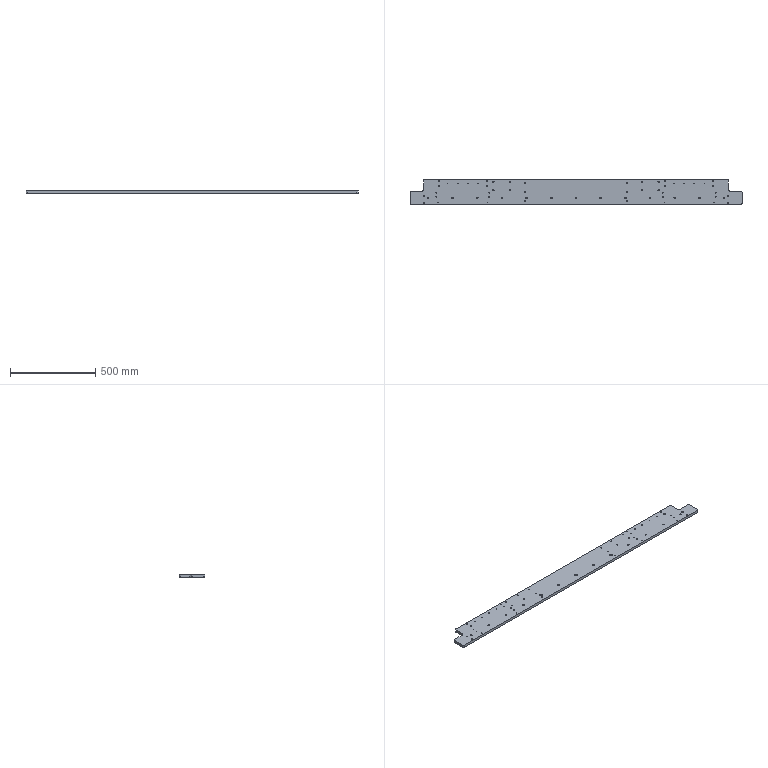Part | SolidWorks | features HoleWzd 12, MirrorPattern 7, LPattern 5, Fillet 3, Cut 1, Extrusion 1 | 1 solid | 175 faces | box 1950 x 150 x 16 mm | volume 4450489 mm3 | cylinder 152 | plane 23 | commonest cylinder face diameters 6.8 x52 5 x32 9 x26 15 x20 3.3 x8 14 x6